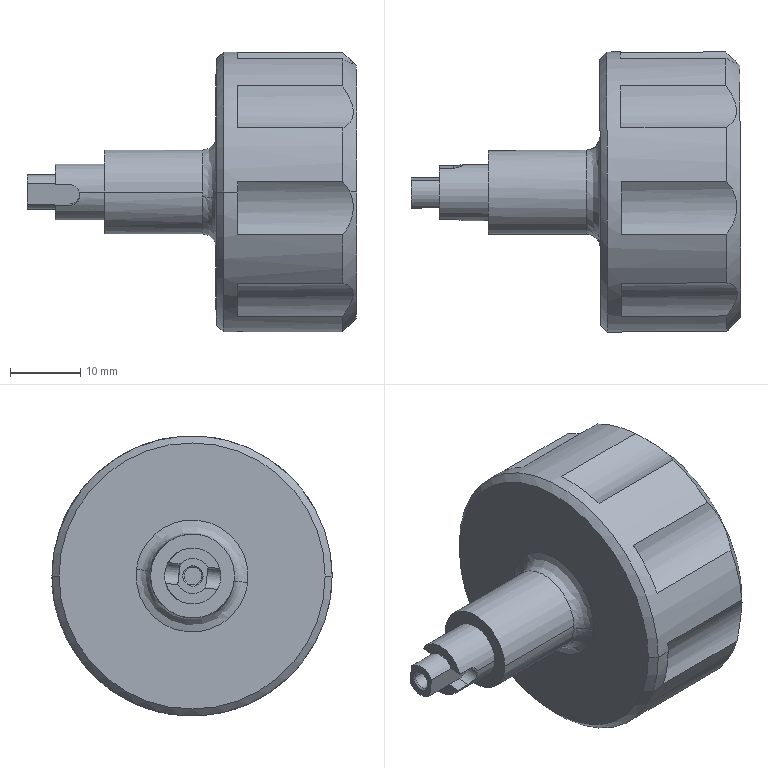Part | SolidWorks | features BaseBody 1 | 1 solid | 52 faces | box 47.088 x 40.019 x 40 mm | volume 26038 mm3 | cylinder 23 | plane 21 | cone 6 | spline 2 | commonest cylinder face diameters 14 x9 3 x4 2.5 x2 5 x2 8 x2 12 x2